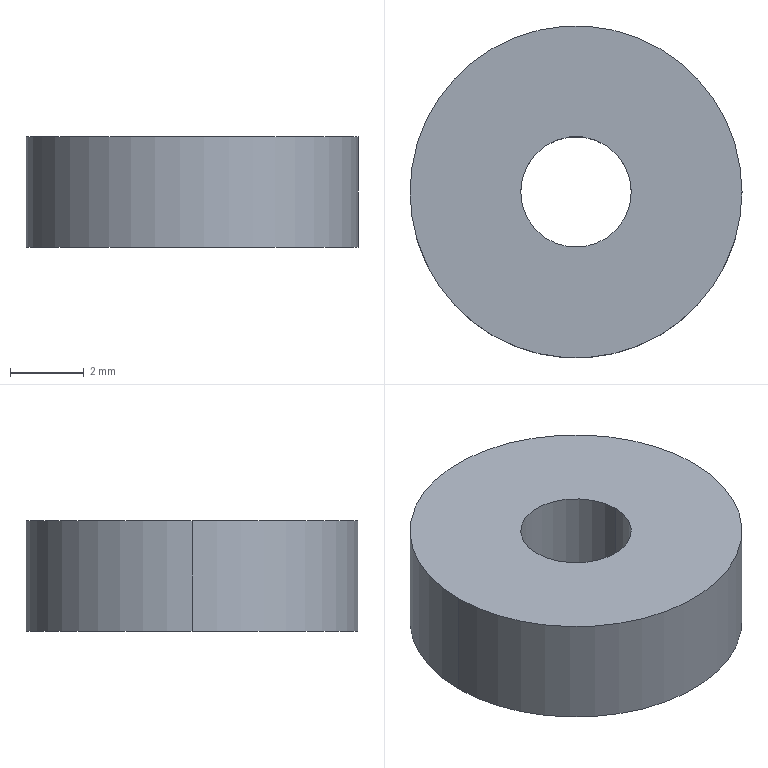Part | NX | features BREP 1 | 1 solid | 6 faces | box 9 x 9 x 3 mm | volume 169.646 mm3 | cylinder 4 | plane 2 | commonest cylinder face diameters 3 x2 9 x2
STEP:
#1=CARTESIAN_POINT('',(-728.215,57.66,3.));
#2=VERTEX_POINT('',#1);
#3=CARTESIAN_POINT('',(-725.215,57.66,3.));
#4=VERTEX_POINT('',#3);
#5=CARTESIAN_POINT('',(-726.715,57.66,3.));
#6=DIRECTION('',(0.,0.,1.));
#7=DIRECTION('',(1.,0.,0.));
#8=AXIS2_PLACEMENT_3D('',#5,#6,#7);
#9=CIRCLE('',#8,1.5);
#10=EDGE_CURVE('',#2,#4,#9,.T.);
#11=ORIENTED_EDGE('',*,*,#10,.T.);
#12=CARTESIAN_POINT('',(-725.215,57.66,0.));
#13=VERTEX_POINT('',#12);
#14=CARTESIAN_POINT('',(-725.215,57.66,3.));
#15=DIRECTION('',(0.,0.,-1.));
#16=VECTOR('',#15,1000.);
#17=LINE('',#14,#16);
#18=EDGE_CURVE('',#4,#13,#17,.T.);
#19=ORIENTED_EDGE('',*,*,#18,.T.);
#20=CARTESIAN_POINT('',(-728.215,57.66,0.));
#21=VERTEX_POINT('',#20);
#22=CARTESIAN_POINT('',(-726.715,57.66,0.));
#23=DIRECTION('',(0.,0.,1.));
#24=DIRECTION('',(1.,0.,0.));
#25=AXIS2_PLACEMENT_3D('',#22,#23,#24);
#26=CIRCLE('',#25,1.5);
#27=EDGE_CURVE('',#21,#13,#26,.T.);
#28=ORIENTED_EDGE('',*,*,#27,.F.);
#29=CARTESIAN_POINT('',(-728.215,57.66,3.));
#30=DIRECTION('',(0.,0.,-1.));
#31=VECTOR('',#30,1000.);
#32=LINE('',#29,#31);
#33=EDGE_CURVE('',#2,#21,#32,.T.);
#34=ORIENTED_EDGE('',*,*,#33,.F.);
#35=EDGE_LOOP('',(#11,#19,#28,#34));
#36=FACE_BOUND('',#35,.T.);
#37=CARTESIAN_POINT('',(-726.715,57.66,3.));
#38=DIRECTION('',(0.,0.,-1.));
#39=DIRECTION('',(-1.,0.,0.));
#40=AXIS2_PLACEMENT_3D('',#37,#38,#39);
#41=CYLINDRICAL_SURFACE('',#40,1.5);
#42=ADVANCED_FACE('',(#36),#41,.F.);
#43=CARTESIAN_POINT('',(-722.215,57.66,3.));
#44=VERTEX_POINT('',#43);
#45=CARTESIAN_POINT('',(-731.215,57.66,3.));
#46=VERTEX_POINT('',#45);
#47=CARTESIAN_POINT('',(-726.715,57.66,3.));
#48=DIRECTION('',(0.,0.,1.));
#49=DIRECTION('',(1.,0.,0.));
#50=AXIS2_PLACEMENT_3D('',#47,#48,#49);
#51=CIRCLE('',#50,4.5);
#52=EDGE_CURVE('',#44,#46,#51,.T.);
#53=ORIENTED_EDGE('',*,*,#52,.F.);
#54=CARTESIAN_POINT('',(-722.215,57.66,0.));
#55=VERTEX_POINT('',#54);
#56=CARTESIAN_POINT('',(-722.215,57.66,3.));
#57=DIRECTION('',(0.,0.,-1.));
#58=VECTOR('',#57,1000.);
#59=LINE('',#56,#58);
#60=EDGE_CURVE('',#44,#55,#59,.T.);
#61=ORIENTED_EDGE('',*,*,#60,.T.);
#62=CARTESIAN_POINT('',(-731.215,57.66,0.));
#63=VERTEX_POINT('',#62);
#64=CARTESIAN_POINT('',(-726.715,57.66,0.));
#65=DIRECTION('',(0.,0.,1.));
#66=DIRECTION('',(1.,0.,0.));
#67=AXIS2_PLACEMENT_3D('',#64,#65,#66);
#68=CIRCLE('',#67,4.5);
#69=EDGE_CURVE('',#55,#63,#68,.T.);
#70=ORIENTED_EDGE('',*,*,#69,.T.);
#71=CARTESIAN_POINT('',(-731.215,57.66,3.));
#72=DIRECTION('',(0.,0.,-1.));
#73=VECTOR('',#72,1000.);
#74=LINE('',#71,#73);
#75=EDGE_CURVE('',#46,#63,#74,.T.);
#76=ORIENTED_EDGE('',*,*,#75,.F.);
#77=EDGE_LOOP('',(#53,#61,#70,#76));
#78=FACE_BOUND('',#77,.T.);
#79=CARTESIAN_POINT('',(-726.715,57.66,3.));
#80=DIRECTION('',(0.,0.,-1.));
#81=DIRECTION('',(-1.,0.,0.));
#82=AXIS2_PLACEMENT_3D('',#79,#80,#81);
#83=CYLINDRICAL_SURFACE('',#82,4.5);
#84=ADVANCED_FACE('',(#78),#83,.T.);
#85=CARTESIAN_POINT('',(-726.715,57.66,3.));
#86=DIRECTION('',(0.,0.,1.));
#87=DIRECTION('',(1.,0.,0.));
#88=AXIS2_PLACEMENT_3D('',#85,#86,#87);
#89=CIRCLE('',#88,4.5);
#90=EDGE_CURVE('',#46,#44,#89,.T.);
#91=ORIENTED_EDGE('',*,*,#90,.T.);
#92=ORIENTED_EDGE('',*,*,#52,.T.);
#93=EDGE_LOOP('',(#91,#92));
#94=FACE_BOUND('',#93,.T.);
#95=ORIENTED_EDGE('',*,*,#10,.F.);
#96=CARTESIAN_POINT('',(-726.715,57.66,3.));
#97=DIRECTION('',(0.,0.,1.));
#98=DIRECTION('',(1.,0.,0.));
#99=AXIS2_PLACEMENT_3D('',#96,#97,#98);
#100=CIRCLE('',#99,1.5);
#101=EDGE_CURVE('',#4,#2,#100,.T.);
#102=ORIENTED_EDGE('',*,*,#101,.F.);
#103=EDGE_LOOP('',(#95,#102));
#104=FACE_BOUND('',#103,.T.);
#105=CARTESIAN_POINT('',(-726.715,57.66,3.));
#106=DIRECTION('',(0.,0.,1.));
#107=DIRECTION('',(1.,0.,0.));
#108=AXIS2_PLACEMENT_3D('',#105,#106,#107);
#109=PLANE('',#108);
#110=ADVANCED_FACE('',(#94,#104),#109,.T.);
#111=CARTESIAN_POINT('',(-726.715,57.66,0.));
#112=DIRECTION('',(0.,0.,1.));
#113=DIRECTION('',(1.,0.,0.));
#114=AXIS2_PLACEMENT_3D('',#111,#112,#113);
#115=CIRCLE('',#114,4.5);
#116=EDGE_CURVE('',#63,#55,#115,.T.);
#117=ORIENTED_EDGE('',*,*,#116,.F.);
#118=ORIENTED_EDGE('',*,*,#69,.F.);
#119=EDGE_LOOP('',(#117,#118));
#120=FACE_BOUND('',#119,.T.);
#121=ORIENTED_EDGE('',*,*,#27,.T.);
#122=CARTESIAN_POINT('',(-726.715,57.66,0.));
#123=DIRECTION('',(0.,0.,1.));
#124=DIRECTION('',(1.,0.,0.));
#125=AXIS2_PLACEMENT_3D('',#122,#123,#124);
#126=CIRCLE('',#125,1.5);
#127=EDGE_CURVE('',#13,#21,#126,.T.);
#128=ORIENTED_EDGE('',*,*,#127,.T.);
#129=EDGE_LOOP('',(#121,#128));
#130=FACE_BOUND('',#129,.T.);
#131=CARTESIAN_POINT('',(-726.715,57.66,0.));
#132=DIRECTION('',(0.,0.,1.));
#133=DIRECTION('',(1.,0.,0.));
#134=AXIS2_PLACEMENT_3D('',#131,#132,#133);
#135=PLANE('',#134);
#136=ADVANCED_FACE('',(#120,#130),#135,.F.);
#137=ORIENTED_EDGE('',*,*,#60,.F.);
#138=ORIENTED_EDGE('',*,*,#90,.F.);
#139=ORIENTED_EDGE('',*,*,#75,.T.);
#140=ORIENTED_EDGE('',*,*,#116,.T.);
#141=EDGE_LOOP('',(#137,#138,#139,#140));
#142=FACE_BOUND('',#141,.T.);
#143=CARTESIAN_POINT('',(-726.715,57.66,3.));
#144=DIRECTION('',(0.,0.,-1.));
#145=DIRECTION('',(-1.,0.,0.));
#146=AXIS2_PLACEMENT_3D('',#143,#144,#145);
#147=CYLINDRICAL_SURFACE('',#146,4.5);
#148=ADVANCED_FACE('',(#142),#147,.T.);
#149=ORIENTED_EDGE('',*,*,#18,.F.);
#150=ORIENTED_EDGE('',*,*,#101,.T.);
#151=ORIENTED_EDGE('',*,*,#33,.T.);
#152=ORIENTED_EDGE('',*,*,#127,.F.);
#153=EDGE_LOOP('',(#149,#150,#151,#152));
#154=FACE_BOUND('',#153,.T.);
#155=CARTESIAN_POINT('',(-726.715,57.66,3.));
#156=DIRECTION('',(0.,0.,-1.));
#157=DIRECTION('',(-1.,0.,0.));
#158=AXIS2_PLACEMENT_3D('',#155,#156,#157);
#159=CYLINDRICAL_SURFACE('',#158,1.5);
#160=ADVANCED_FACE('',(#154),#159,.F.);
#161=CLOSED_SHELL('',(#42,#84,#110,#136,#148,#160));
#162=MANIFOLD_SOLID_BREP('',#161);
#163=(LENGTH_UNIT()NAMED_UNIT(*)SI_UNIT(.MILLI.,.METRE.));
#164=UNCERTAINTY_MEASURE_WITH_UNIT(LENGTH_MEASURE(0.00001),#163,'','');
#165=(NAMED_UNIT(*)PLANE_ANGLE_UNIT()SI_UNIT($,.RADIAN.));
#166=(NAMED_UNIT(*)SI_UNIT($,.STERADIAN.)SOLID_ANGLE_UNIT());
#167=(GEOMETRIC_REPRESENTATION_CONTEXT(3)GLOBAL_UNCERTAINTY_ASSIGNED_CONTEXT((#164))GLOBAL_UNIT_ASSIGNED_CONTEXT((#163,#165,#166))REPRESENTATION_CONTEXT('',''));
#168=ADVANCED_BREP_SHAPE_REPRESENTATION('',(#162),#167);